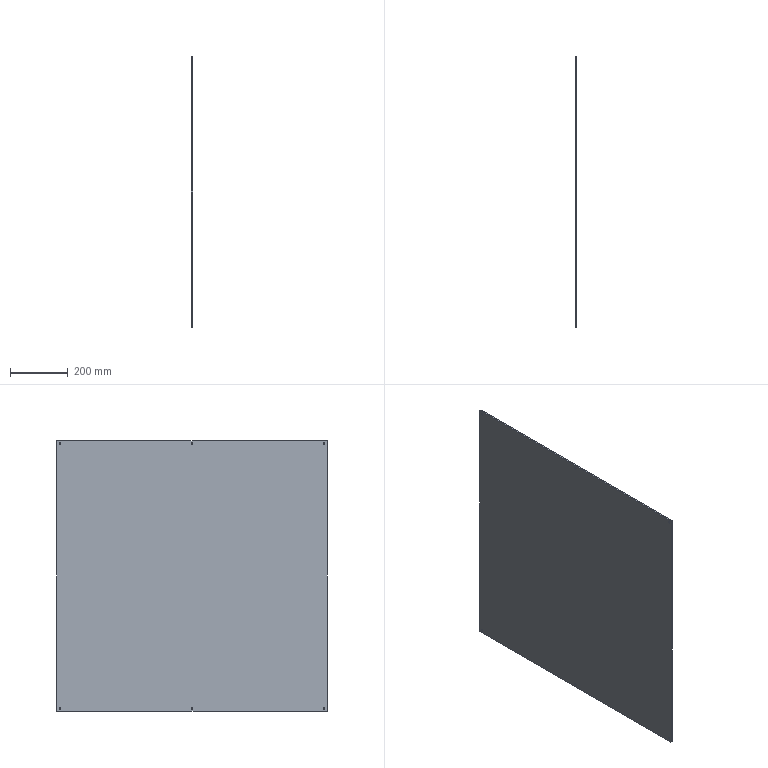Part | SolidWorks | features Chamfer 1, Extrusion 1, ICE 1 | 1 solid | 22 faces | box 5 x 937 x 938 mm | volume 4393672 mm3 | cylinder 12 | plane 10 | commonest cylinder face diameters 6 x12
STEP:
#1=CARTESIAN_POINT('',(5.,0.,-461.));
#2=VERTEX_POINT('',#1);
#3=CARTESIAN_POINT('',(5.,0.,-455.));
#4=VERTEX_POINT('',#3);
#5=CARTESIAN_POINT('',(5.,0.,-458.));
#6=DIRECTION('',(-1.,0.,0.));
#7=DIRECTION('',(0.,0.,1.));
#8=AXIS2_PLACEMENT_3D('',#5,#6,#7);
#9=CIRCLE('',#8,3.);
#10=EDGE_CURVE('',#2,#4,#9,.T.);
#11=ORIENTED_EDGE('',*,*,#10,.F.);
#12=CARTESIAN_POINT('',(0.,0.,-461.));
#13=VERTEX_POINT('',#12);
#14=CARTESIAN_POINT('',(5.,0.,-461.));
#15=DIRECTION('',(-1.,0.,0.));
#16=VECTOR('',#15,1000.);
#17=LINE('',#14,#16);
#18=EDGE_CURVE('',#2,#13,#17,.T.);
#19=ORIENTED_EDGE('',*,*,#18,.T.);
#20=CARTESIAN_POINT('',(0.,0.,-455.));
#21=VERTEX_POINT('',#20);
#22=CARTESIAN_POINT('',(0.,0.,-458.));
#23=DIRECTION('',(-1.,0.,0.));
#24=DIRECTION('',(0.,0.,1.));
#25=AXIS2_PLACEMENT_3D('',#22,#23,#24);
#26=CIRCLE('',#25,3.);
#27=EDGE_CURVE('',#13,#21,#26,.T.);
#28=ORIENTED_EDGE('',*,*,#27,.T.);
#29=CARTESIAN_POINT('',(5.,0.,-455.));
#30=DIRECTION('',(-1.,0.,0.));
#31=VECTOR('',#30,1000.);
#32=LINE('',#29,#31);
#33=EDGE_CURVE('',#4,#21,#32,.T.);
#34=ORIENTED_EDGE('',*,*,#33,.F.);
#35=EDGE_LOOP('',(#11,#19,#28,#34));
#36=FACE_OUTER_BOUND('',#35,.T.);
#37=CARTESIAN_POINT('',(5.,0.,-458.));
#38=DIRECTION('',(-1.,0.,0.));
#39=DIRECTION('',(0.,0.,1.));
#40=AXIS2_PLACEMENT_3D('',#37,#38,#39);
#41=CYLINDRICAL_SURFACE('',#40,3.);
#42=ADVANCED_FACE('',(#36),#41,.F.);
#43=CARTESIAN_POINT('',(5.,0.,455.));
#44=VERTEX_POINT('',#43);
#45=CARTESIAN_POINT('',(5.,0.,461.));
#46=VERTEX_POINT('',#45);
#47=CARTESIAN_POINT('',(5.,0.,458.));
#48=DIRECTION('',(-1.,0.,0.));
#49=DIRECTION('',(0.,0.,1.));
#50=AXIS2_PLACEMENT_3D('',#47,#48,#49);
#51=CIRCLE('',#50,3.);
#52=EDGE_CURVE('',#44,#46,#51,.T.);
#53=ORIENTED_EDGE('',*,*,#52,.F.);
#54=CARTESIAN_POINT('',(0.,0.,455.));
#55=VERTEX_POINT('',#54);
#56=CARTESIAN_POINT('',(5.,0.,455.));
#57=DIRECTION('',(-1.,0.,0.));
#58=VECTOR('',#57,1000.);
#59=LINE('',#56,#58);
#60=EDGE_CURVE('',#44,#55,#59,.T.);
#61=ORIENTED_EDGE('',*,*,#60,.T.);
#62=CARTESIAN_POINT('',(0.,0.,461.));
#63=VERTEX_POINT('',#62);
#64=CARTESIAN_POINT('',(0.,0.,458.));
#65=DIRECTION('',(-1.,0.,0.));
#66=DIRECTION('',(0.,0.,1.));
#67=AXIS2_PLACEMENT_3D('',#64,#65,#66);
#68=CIRCLE('',#67,3.);
#69=EDGE_CURVE('',#55,#63,#68,.T.);
#70=ORIENTED_EDGE('',*,*,#69,.T.);
#71=CARTESIAN_POINT('',(5.,0.,461.));
#72=DIRECTION('',(-1.,0.,0.));
#73=VECTOR('',#72,1000.);
#74=LINE('',#71,#73);
#75=EDGE_CURVE('',#46,#63,#74,.T.);
#76=ORIENTED_EDGE('',*,*,#75,.F.);
#77=EDGE_LOOP('',(#53,#61,#70,#76));
#78=FACE_OUTER_BOUND('',#77,.T.);
#79=CARTESIAN_POINT('',(5.,0.,458.));
#80=DIRECTION('',(-1.,0.,0.));
#81=DIRECTION('',(0.,0.,1.));
#82=AXIS2_PLACEMENT_3D('',#79,#80,#81);
#83=CYLINDRICAL_SURFACE('',#82,3.);
#84=ADVANCED_FACE('',(#78),#83,.F.);
#85=CARTESIAN_POINT('',(5.,457.5,455.));
#86=VERTEX_POINT('',#85);
#87=CARTESIAN_POINT('',(5.,457.5,461.));
#88=VERTEX_POINT('',#87);
#89=CARTESIAN_POINT('',(5.,457.5,458.));
#90=DIRECTION('',(-1.,0.,0.));
#91=DIRECTION('',(0.,0.,-1.));
#92=AXIS2_PLACEMENT_3D('',#89,#90,#91);
#93=CIRCLE('',#92,3.);
#94=EDGE_CURVE('',#86,#88,#93,.T.);
#95=ORIENTED_EDGE('',*,*,#94,.F.);
#96=CARTESIAN_POINT('',(0.,457.5,455.));
#97=VERTEX_POINT('',#96);
#98=CARTESIAN_POINT('',(5.,457.5,455.));
#99=DIRECTION('',(-1.,0.,0.));
#100=VECTOR('',#99,1000.);
#101=LINE('',#98,#100);
#102=EDGE_CURVE('',#86,#97,#101,.T.);
#103=ORIENTED_EDGE('',*,*,#102,.T.);
#104=CARTESIAN_POINT('',(0.,457.5,461.));
#105=VERTEX_POINT('',#104);
#106=CARTESIAN_POINT('',(0.,457.5,458.));
#107=DIRECTION('',(-1.,0.,0.));
#108=DIRECTION('',(0.,0.,-1.));
#109=AXIS2_PLACEMENT_3D('',#106,#107,#108);
#110=CIRCLE('',#109,3.);
#111=EDGE_CURVE('',#97,#105,#110,.T.);
#112=ORIENTED_EDGE('',*,*,#111,.T.);
#113=CARTESIAN_POINT('',(5.,457.5,461.));
#114=DIRECTION('',(-1.,0.,0.));
#115=VECTOR('',#114,1000.);
#116=LINE('',#113,#115);
#117=EDGE_CURVE('',#88,#105,#116,.T.);
#118=ORIENTED_EDGE('',*,*,#117,.F.);
#119=EDGE_LOOP('',(#95,#103,#112,#118));
#120=FACE_OUTER_BOUND('',#119,.T.);
#121=CARTESIAN_POINT('',(5.,457.5,458.));
#122=DIRECTION('',(-1.,0.,0.));
#123=DIRECTION('',(0.,0.,1.));
#124=AXIS2_PLACEMENT_3D('',#121,#122,#123);
#125=CYLINDRICAL_SURFACE('',#124,3.);
#126=ADVANCED_FACE('',(#120),#125,.F.);
#127=CARTESIAN_POINT('',(5.,-457.5,455.));
#128=VERTEX_POINT('',#127);
#129=CARTESIAN_POINT('',(5.,-457.5,461.));
#130=VERTEX_POINT('',#129);
#131=CARTESIAN_POINT('',(5.,-457.5,458.));
#132=DIRECTION('',(-1.,0.,0.));
#133=DIRECTION('',(0.,0.,1.));
#134=AXIS2_PLACEMENT_3D('',#131,#132,#133);
#135=CIRCLE('',#134,3.);
#136=EDGE_CURVE('',#128,#130,#135,.T.);
#137=ORIENTED_EDGE('',*,*,#136,.F.);
#138=CARTESIAN_POINT('',(0.,-457.5,455.));
#139=VERTEX_POINT('',#138);
#140=CARTESIAN_POINT('',(5.,-457.5,455.));
#141=DIRECTION('',(-1.,0.,0.));
#142=VECTOR('',#141,1000.);
#143=LINE('',#140,#142);
#144=EDGE_CURVE('',#128,#139,#143,.T.);
#145=ORIENTED_EDGE('',*,*,#144,.T.);
#146=CARTESIAN_POINT('',(0.,-457.5,461.));
#147=VERTEX_POINT('',#146);
#148=CARTESIAN_POINT('',(0.,-457.5,458.));
#149=DIRECTION('',(-1.,0.,0.));
#150=DIRECTION('',(0.,0.,1.));
#151=AXIS2_PLACEMENT_3D('',#148,#149,#150);
#152=CIRCLE('',#151,3.);
#153=EDGE_CURVE('',#139,#147,#152,.T.);
#154=ORIENTED_EDGE('',*,*,#153,.T.);
#155=CARTESIAN_POINT('',(5.,-457.5,461.));
#156=DIRECTION('',(-1.,0.,0.));
#157=VECTOR('',#156,1000.);
#158=LINE('',#155,#157);
#159=EDGE_CURVE('',#130,#147,#158,.T.);
#160=ORIENTED_EDGE('',*,*,#159,.F.);
#161=EDGE_LOOP('',(#137,#145,#154,#160));
#162=FACE_OUTER_BOUND('',#161,.T.);
#163=CARTESIAN_POINT('',(5.,-457.5,458.));
#164=DIRECTION('',(-1.,0.,0.));
#165=DIRECTION('',(0.,0.,1.));
#166=AXIS2_PLACEMENT_3D('',#163,#164,#165);
#167=CYLINDRICAL_SURFACE('',#166,3.);
#168=ADVANCED_FACE('',(#162),#167,.F.);
#169=CARTESIAN_POINT('',(5.,-457.5,-461.));
#170=VERTEX_POINT('',#169);
#171=CARTESIAN_POINT('',(5.,-457.5,-455.));
#172=VERTEX_POINT('',#171);
#173=CARTESIAN_POINT('',(5.,-457.5,-458.));
#174=DIRECTION('',(-1.,0.,0.));
#175=DIRECTION('',(0.,0.,-1.));
#176=AXIS2_PLACEMENT_3D('',#173,#174,#175);
#177=CIRCLE('',#176,3.);
#178=EDGE_CURVE('',#170,#172,#177,.T.);
#179=ORIENTED_EDGE('',*,*,#178,.F.);
#180=CARTESIAN_POINT('',(0.,-457.5,-461.));
#181=VERTEX_POINT('',#180);
#182=CARTESIAN_POINT('',(5.,-457.5,-461.));
#183=DIRECTION('',(-1.,0.,0.));
#184=VECTOR('',#183,1000.);
#185=LINE('',#182,#184);
#186=EDGE_CURVE('',#170,#181,#185,.T.);
#187=ORIENTED_EDGE('',*,*,#186,.T.);
#188=CARTESIAN_POINT('',(0.,-457.5,-455.));
#189=VERTEX_POINT('',#188);
#190=CARTESIAN_POINT('',(0.,-457.5,-458.));
#191=DIRECTION('',(-1.,0.,0.));
#192=DIRECTION('',(0.,0.,-1.));
#193=AXIS2_PLACEMENT_3D('',#190,#191,#192);
#194=CIRCLE('',#193,3.);
#195=EDGE_CURVE('',#181,#189,#194,.T.);
#196=ORIENTED_EDGE('',*,*,#195,.T.);
#197=CARTESIAN_POINT('',(5.,-457.5,-455.));
#198=DIRECTION('',(-1.,0.,0.));
#199=VECTOR('',#198,1000.);
#200=LINE('',#197,#199);
#201=EDGE_CURVE('',#172,#189,#200,.T.);
#202=ORIENTED_EDGE('',*,*,#201,.F.);
#203=EDGE_LOOP('',(#179,#187,#196,#202));
#204=FACE_OUTER_BOUND('',#203,.T.);
#205=CARTESIAN_POINT('',(5.,-457.5,-458.));
#206=DIRECTION('',(-1.,0.,0.));
#207=DIRECTION('',(0.,0.,1.));
#208=AXIS2_PLACEMENT_3D('',#205,#206,#207);
#209=CYLINDRICAL_SURFACE('',#208,3.);
#210=ADVANCED_FACE('',(#204),#209,.F.);
#211=CARTESIAN_POINT('',(5.,457.5,-461.));
#212=VERTEX_POINT('',#211);
#213=CARTESIAN_POINT('',(5.,457.5,-455.));
#214=VERTEX_POINT('',#213);
#215=CARTESIAN_POINT('',(5.,457.5,-458.));
#216=DIRECTION('',(-1.,0.,0.));
#217=DIRECTION('',(0.,0.,1.));
#218=AXIS2_PLACEMENT_3D('',#215,#216,#217);
#219=CIRCLE('',#218,3.);
#220=EDGE_CURVE('',#212,#214,#219,.T.);
#221=ORIENTED_EDGE('',*,*,#220,.F.);
#222=CARTESIAN_POINT('',(0.,457.5,-461.));
#223=VERTEX_POINT('',#222);
#224=CARTESIAN_POINT('',(5.,457.5,-461.));
#225=DIRECTION('',(-1.,0.,0.));
#226=VECTOR('',#225,1000.);
#227=LINE('',#224,#226);
#228=EDGE_CURVE('',#212,#223,#227,.T.);
#229=ORIENTED_EDGE('',*,*,#228,.T.);
#230=CARTESIAN_POINT('',(0.,457.5,-455.));
#231=VERTEX_POINT('',#230);
#232=CARTESIAN_POINT('',(0.,457.5,-458.));
#233=DIRECTION('',(-1.,0.,0.));
#234=DIRECTION('',(0.,0.,1.));
#235=AXIS2_PLACEMENT_3D('',#232,#233,#234);
#236=CIRCLE('',#235,3.);
#237=EDGE_CURVE('',#223,#231,#236,.T.);
#238=ORIENTED_EDGE('',*,*,#237,.T.);
#239=CARTESIAN_POINT('',(5.,457.5,-455.));
#240=DIRECTION('',(-1.,0.,0.));
#241=VECTOR('',#240,1000.);
#242=LINE('',#239,#241);
#243=EDGE_CURVE('',#214,#231,#242,.T.);
#244=ORIENTED_EDGE('',*,*,#243,.F.);
#245=EDGE_LOOP('',(#221,#229,#238,#244));
#246=FACE_OUTER_BOUND('',#245,.T.);
#247=CARTESIAN_POINT('',(5.,457.5,-458.));
#248=DIRECTION('',(-1.,0.,0.));
#249=DIRECTION('',(0.,0.,1.));
#250=AXIS2_PLACEMENT_3D('',#247,#248,#249);
#251=CYLINDRICAL_SURFACE('',#250,3.);
#252=ADVANCED_FACE('',(#246),#251,.F.);
#253=CARTESIAN_POINT('',(0.,467.5,469.));
#254=VERTEX_POINT('',#253);
#255=CARTESIAN_POINT('',(0.,-467.5,469.));
#256=VERTEX_POINT('',#255);
#257=CARTESIAN_POINT('',(0.,468.5,469.));
#258=DIRECTION('',(0.,-1.,0.));
#259=VECTOR('',#258,1000.);
#260=LINE('',#257,#259);
#261=EDGE_CURVE('',#254,#256,#260,.T.);
#262=ORIENTED_EDGE('',*,*,#261,.T.);
#263=CARTESIAN_POINT('',(5.,-467.5,469.));
#264=VERTEX_POINT('',#263);
#265=CARTESIAN_POINT('',(5.,-467.5,469.));
#266=DIRECTION('',(1.,0.,0.));
#267=VECTOR('',#266,1000.);
#268=LINE('',#265,#267);
#269=EDGE_CURVE('',#256,#264,#268,.T.);
#270=ORIENTED_EDGE('',*,*,#269,.T.);
#271=CARTESIAN_POINT('',(5.,467.5,469.));
#272=VERTEX_POINT('',#271);
#273=CARTESIAN_POINT('',(5.,468.5,469.));
#274=DIRECTION('',(0.,-1.,0.));
#275=VECTOR('',#274,1000.);
#276=LINE('',#273,#275);
#277=EDGE_CURVE('',#272,#264,#276,.T.);
#278=ORIENTED_EDGE('',*,*,#277,.F.);
#279=CARTESIAN_POINT('',(5.,467.5,469.));
#280=DIRECTION('',(-1.,0.,0.));
#281=VECTOR('',#280,1000.);
#282=LINE('',#279,#281);
#283=EDGE_CURVE('',#272,#254,#282,.T.);
#284=ORIENTED_EDGE('',*,*,#283,.T.);
#285=EDGE_LOOP('',(#262,#270,#278,#284));
#286=FACE_OUTER_BOUND('',#285,.T.);
#287=CARTESIAN_POINT('',(5.,468.5,469.));
#288=DIRECTION('',(0.,0.,-1.));
#289=DIRECTION('',(0.,1.,0.));
#290=AXIS2_PLACEMENT_3D('',#287,#288,#289);
#291=PLANE('',#290);
#292=ADVANCED_FACE('',(#286),#291,.F.);
#293=CARTESIAN_POINT('',(0.,-468.5,468.));
#294=VERTEX_POINT('',#293);
#295=CARTESIAN_POINT('',(0.,-468.5,-468.));
#296=VERTEX_POINT('',#295);
#297=CARTESIAN_POINT('',(0.,-468.5,-469.));
#298=DIRECTION('',(0.,0.,-1.));
#299=VECTOR('',#298,1000.);
#300=LINE('',#297,#299);
#301=EDGE_CURVE('',#294,#296,#300,.T.);
#302=ORIENTED_EDGE('',*,*,#301,.T.);
#303=CARTESIAN_POINT('',(5.,-468.5,-468.));
#304=VERTEX_POINT('',#303);
#305=CARTESIAN_POINT('',(5.,-468.5,-468.));
#306=DIRECTION('',(1.,0.,0.));
#307=VECTOR('',#306,1000.);
#308=LINE('',#305,#307);
#309=EDGE_CURVE('',#296,#304,#308,.T.);
#310=ORIENTED_EDGE('',*,*,#309,.T.);
#311=CARTESIAN_POINT('',(5.,-468.5,468.));
#312=VERTEX_POINT('',#311);
#313=CARTESIAN_POINT('',(5.,-468.5,-469.));
#314=DIRECTION('',(0.,0.,-1.));
#315=VECTOR('',#314,1000.);
#316=LINE('',#313,#315);
#317=EDGE_CURVE('',#312,#304,#316,.T.);
#318=ORIENTED_EDGE('',*,*,#317,.F.);
#319=CARTESIAN_POINT('',(5.,-468.5,468.));
#320=DIRECTION('',(-1.,0.,0.));
#321=VECTOR('',#320,1000.);
#322=LINE('',#319,#321);
#323=EDGE_CURVE('',#312,#294,#322,.T.);
#324=ORIENTED_EDGE('',*,*,#323,.T.);
#325=EDGE_LOOP('',(#302,#310,#318,#324));
#326=FACE_OUTER_BOUND('',#325,.T.);
#327=CARTESIAN_POINT('',(5.,-468.5,-469.));
#328=DIRECTION('',(0.,1.,0.));
#329=DIRECTION('',(0.,0.,1.));
#330=AXIS2_PLACEMENT_3D('',#327,#328,#329);
#331=PLANE('',#330);
#332=ADVANCED_FACE('',(#326),#331,.F.);
#333=CARTESIAN_POINT('',(5.,-467.5,-469.));
#334=VERTEX_POINT('',#333);
#335=CARTESIAN_POINT('',(5.,467.5,-469.));
#336=VERTEX_POINT('',#335);
#337=CARTESIAN_POINT('',(5.,468.5,-469.));
#338=DIRECTION('',(0.,1.,0.));
#339=VECTOR('',#338,1000.);
#340=LINE('',#337,#339);
#341=EDGE_CURVE('',#334,#336,#340,.T.);
#342=ORIENTED_EDGE('',*,*,#341,.F.);
#343=CARTESIAN_POINT('',(0.,-467.5,-469.));
#344=VERTEX_POINT('',#343);
#345=CARTESIAN_POINT('',(5.,-467.5,-469.));
#346=DIRECTION('',(-1.,0.,0.));
#347=VECTOR('',#346,1000.);
#348=LINE('',#345,#347);
#349=EDGE_CURVE('',#334,#344,#348,.T.);
#350=ORIENTED_EDGE('',*,*,#349,.T.);
#351=CARTESIAN_POINT('',(0.,467.5,-469.));
#352=VERTEX_POINT('',#351);
#353=CARTESIAN_POINT('',(0.,468.5,-469.));
#354=DIRECTION('',(0.,1.,0.));
#355=VECTOR('',#354,1000.);
#356=LINE('',#353,#355);
#357=EDGE_CURVE('',#344,#352,#356,.T.);
#358=ORIENTED_EDGE('',*,*,#357,.T.);
#359=CARTESIAN_POINT('',(5.,467.5,-469.));
#360=DIRECTION('',(1.,0.,0.));
#361=VECTOR('',#360,1000.);
#362=LINE('',#359,#361);
#363=EDGE_CURVE('',#352,#336,#362,.T.);
#364=ORIENTED_EDGE('',*,*,#363,.T.);
#365=EDGE_LOOP('',(#342,#350,#358,#364));
#366=FACE_OUTER_BOUND('',#365,.T.);
#367=CARTESIAN_POINT('',(5.,468.5,-469.));
#368=DIRECTION('',(0.,0.,1.));
#369=DIRECTION('',(0.,-1.,0.));
#370=AXIS2_PLACEMENT_3D('',#367,#368,#369);
#371=PLANE('',#370);
#372=ADVANCED_FACE('',(#366),#371,.F.);
#373=CARTESIAN_POINT('',(5.,468.5,-468.));
#374=VERTEX_POINT('',#373);
#375=CARTESIAN_POINT('',(5.,468.5,468.));
#376=VERTEX_POINT('',#375);
#377=CARTESIAN_POINT('',(5.,468.5,-469.));
#378=DIRECTION('',(0.,0.,1.));
#379=VECTOR('',#378,1000.);
#380=LINE('',#377,#379);
#381=EDGE_CURVE('',#374,#376,#380,.T.);
#382=ORIENTED_EDGE('',*,*,#381,.F.);
#383=CARTESIAN_POINT('',(0.,468.5,-468.));
#384=VERTEX_POINT('',#383);
#385=CARTESIAN_POINT('',(5.,468.5,-468.));
#386=DIRECTION('',(-1.,0.,0.));
#387=VECTOR('',#386,1000.);
#388=LINE('',#385,#387);
#389=EDGE_CURVE('',#374,#384,#388,.T.);
#390=ORIENTED_EDGE('',*,*,#389,.T.);
#391=CARTESIAN_POINT('',(0.,468.5,468.));
#392=VERTEX_POINT('',#391);
#393=CARTESIAN_POINT('',(0.,468.5,-469.));
#394=DIRECTION('',(0.,0.,1.));
#395=VECTOR('',#394,1000.);
#396=LINE('',#393,#395);
#397=EDGE_CURVE('',#384,#392,#396,.T.);
#398=ORIENTED_EDGE('',*,*,#397,.T.);
#399=CARTESIAN_POINT('',(5.,468.5,468.));
#400=DIRECTION('',(1.,0.,0.));
#401=VECTOR('',#400,1000.);
#402=LINE('',#399,#401);
#403=EDGE_CURVE('',#392,#376,#402,.T.);
#404=ORIENTED_EDGE('',*,*,#403,.T.);
#405=EDGE_LOOP('',(#382,#390,#398,#404));
#406=FACE_OUTER_BOUND('',#405,.T.);
#407=CARTESIAN_POINT('',(5.,468.5,-469.));
#408=DIRECTION('',(0.,-1.,0.));
#409=DIRECTION('',(0.,0.,-1.));
#410=AXIS2_PLACEMENT_3D('',#407,#408,#409);
#411=PLANE('',#410);
#412=ADVANCED_FACE('',(#406),#411,.F.);
#413=CARTESIAN_POINT('',(5.,0.,-458.));
#414=DIRECTION('',(-1.,0.,0.));
#415=DIRECTION('',(0.,0.,1.));
#416=AXIS2_PLACEMENT_3D('',#413,#414,#415);
#417=CIRCLE('',#416,3.);
#418=EDGE_CURVE('',#4,#2,#417,.T.);
#419=ORIENTED_EDGE('',*,*,#418,.T.);
#420=ORIENTED_EDGE('',*,*,#10,.T.);
#421=EDGE_LOOP('',(#419,#420));
#422=FACE_BOUND('',#421,.T.);
#423=CARTESIAN_POINT('',(5.,0.,458.));
#424=DIRECTION('',(-1.,0.,0.));
#425=DIRECTION('',(0.,0.,1.));
#426=AXIS2_PLACEMENT_3D('',#423,#424,#425);
#427=CIRCLE('',#426,3.);
#428=EDGE_CURVE('',#46,#44,#427,.T.);
#429=ORIENTED_EDGE('',*,*,#428,.T.);
#430=ORIENTED_EDGE('',*,*,#52,.T.);
#431=EDGE_LOOP('',(#429,#430));
#432=FACE_BOUND('',#431,.T.);
#433=CARTESIAN_POINT('',(5.,457.5,458.));
#434=DIRECTION('',(-1.,0.,0.));
#435=DIRECTION('',(0.,0.,-1.));
#436=AXIS2_PLACEMENT_3D('',#433,#434,#435);
#437=CIRCLE('',#436,3.);
#438=EDGE_CURVE('',#88,#86,#437,.T.);
#439=ORIENTED_EDGE('',*,*,#438,.T.);
#440=ORIENTED_EDGE('',*,*,#94,.T.);
#441=EDGE_LOOP('',(#439,#440));
#442=FACE_BOUND('',#441,.T.);
#443=CARTESIAN_POINT('',(5.,-457.5,458.));
#444=DIRECTION('',(-1.,0.,0.));
#445=DIRECTION('',(0.,0.,1.));
#446=AXIS2_PLACEMENT_3D('',#443,#444,#445);
#447=CIRCLE('',#446,3.);
#448=EDGE_CURVE('',#130,#128,#447,.T.);
#449=ORIENTED_EDGE('',*,*,#448,.T.);
#450=ORIENTED_EDGE('',*,*,#136,.T.);
#451=EDGE_LOOP('',(#449,#450));
#452=FACE_BOUND('',#451,.T.);
#453=CARTESIAN_POINT('',(5.,-457.5,-458.));
#454=DIRECTION('',(-1.,0.,0.));
#455=DIRECTION('',(0.,0.,-1.));
#456=AXIS2_PLACEMENT_3D('',#453,#454,#455);
#457=CIRCLE('',#456,3.);
#458=EDGE_CURVE('',#172,#170,#457,.T.);
#459=ORIENTED_EDGE('',*,*,#458,.T.);
#460=ORIENTED_EDGE('',*,*,#178,.T.);
#461=EDGE_LOOP('',(#459,#460));
#462=FACE_BOUND('',#461,.T.);
#463=CARTESIAN_POINT('',(5.,457.5,-458.));
#464=DIRECTION('',(-1.,0.,0.));
#465=DIRECTION('',(0.,0.,1.));
#466=AXIS2_PLACEMENT_3D('',#463,#464,#465);
#467=CIRCLE('',#466,3.);
#468=EDGE_CURVE('',#214,#212,#467,.T.);
#469=ORIENTED_EDGE('',*,*,#468,.T.);
#470=ORIENTED_EDGE('',*,*,#220,.T.);
#471=EDGE_LOOP('',(#469,#470));
#472=FACE_BOUND('',#471,.T.);
#473=ORIENTED_EDGE('',*,*,#317,.T.);
#474=CARTESIAN_POINT('',(5.,-467.5,-469.));
#475=DIRECTION('',(0.,0.7071,-0.7071));
#476=VECTOR('',#475,1000.);
#477=LINE('',#474,#476);
#478=EDGE_CURVE('',#304,#334,#477,.T.);
#479=ORIENTED_EDGE('',*,*,#478,.T.);
#480=ORIENTED_EDGE('',*,*,#341,.T.);
#481=CARTESIAN_POINT('',(5.,468.5,-468.));
#482=DIRECTION('',(0.,0.7071,0.7071));
#483=VECTOR('',#482,1000.);
#484=LINE('',#481,#483);
#485=EDGE_CURVE('',#336,#374,#484,.T.);
#486=ORIENTED_EDGE('',*,*,#485,.T.);
#487=ORIENTED_EDGE('',*,*,#381,.T.);
#488=CARTESIAN_POINT('',(5.,467.5,469.));
#489=DIRECTION('',(0.,-0.7071,0.7071));
#490=VECTOR('',#489,1000.);
#491=LINE('',#488,#490);
#492=EDGE_CURVE('',#376,#272,#491,.T.);
#493=ORIENTED_EDGE('',*,*,#492,.T.);
#494=ORIENTED_EDGE('',*,*,#277,.T.);
#495=CARTESIAN_POINT('',(5.,-468.5,468.));
#496=DIRECTION('',(0.,-0.7071,-0.7071));
#497=VECTOR('',#496,1000.);
#498=LINE('',#495,#497);
#499=EDGE_CURVE('',#264,#312,#498,.T.);
#500=ORIENTED_EDGE('',*,*,#499,.T.);
#501=EDGE_LOOP('',(#473,#479,#480,#486,#487,#493,#494,#500));
#502=FACE_OUTER_BOUND('',#501,.T.);
#503=CARTESIAN_POINT('',(5.,-468.5,469.));
#504=DIRECTION('',(-1.,0.,0.));
#505=DIRECTION('',(0.,0.,1.));
#506=AXIS2_PLACEMENT_3D('',#503,#504,#505);
#507=PLANE('',#506);
#508=ADVANCED_FACE('',(#422,#432,#442,#452,#462,#472,#502),#507,.F.);
#509=CARTESIAN_POINT('',(0.,0.,-458.));
#510=DIRECTION('',(-1.,0.,0.));
#511=DIRECTION('',(0.,0.,1.));
#512=AXIS2_PLACEMENT_3D('',#509,#510,#511);
#513=CIRCLE('',#512,3.);
#514=EDGE_CURVE('',#21,#13,#513,.T.);
#515=ORIENTED_EDGE('',*,*,#514,.F.);
#516=ORIENTED_EDGE('',*,*,#27,.F.);
#517=EDGE_LOOP('',(#515,#516));
#518=FACE_BOUND('',#517,.T.);
#519=CARTESIAN_POINT('',(0.,0.,458.));
#520=DIRECTION('',(-1.,0.,0.));
#521=DIRECTION('',(0.,0.,1.));
#522=AXIS2_PLACEMENT_3D('',#519,#520,#521);
#523=CIRCLE('',#522,3.);
#524=EDGE_CURVE('',#63,#55,#523,.T.);
#525=ORIENTED_EDGE('',*,*,#524,.F.);
#526=ORIENTED_EDGE('',*,*,#69,.F.);
#527=EDGE_LOOP('',(#525,#526));
#528=FACE_BOUND('',#527,.T.);
#529=CARTESIAN_POINT('',(0.,457.5,458.));
#530=DIRECTION('',(-1.,0.,0.));
#531=DIRECTION('',(0.,0.,-1.));
#532=AXIS2_PLACEMENT_3D('',#529,#530,#531);
#533=CIRCLE('',#532,3.);
#534=EDGE_CURVE('',#105,#97,#533,.T.);
#535=ORIENTED_EDGE('',*,*,#534,.F.);
#536=ORIENTED_EDGE('',*,*,#111,.F.);
#537=EDGE_LOOP('',(#535,#536));
#538=FACE_BOUND('',#537,.T.);
#539=CARTESIAN_POINT('',(0.,-457.5,458.));
#540=DIRECTION('',(-1.,0.,0.));
#541=DIRECTION('',(0.,0.,1.));
#542=AXIS2_PLACEMENT_3D('',#539,#540,#541);
#543=CIRCLE('',#542,3.);
#544=EDGE_CURVE('',#147,#139,#543,.T.);
#545=ORIENTED_EDGE('',*,*,#544,.F.);
#546=ORIENTED_EDGE('',*,*,#153,.F.);
#547=EDGE_LOOP('',(#545,#546));
#548=FACE_BOUND('',#547,.T.);
#549=CARTESIAN_POINT('',(0.,-457.5,-458.));
#550=DIRECTION('',(-1.,0.,0.));
#551=DIRECTION('',(0.,0.,-1.));
#552=AXIS2_PLACEMENT_3D('',#549,#550,#551);
#553=CIRCLE('',#552,3.);
#554=EDGE_CURVE('',#189,#181,#553,.T.);
#555=ORIENTED_EDGE('',*,*,#554,.F.);
#556=ORIENTED_EDGE('',*,*,#195,.F.);
#557=EDGE_LOOP('',(#555,#556));
#558=FACE_BOUND('',#557,.T.);
#559=CARTESIAN_POINT('',(0.,457.5,-458.));
#560=DIRECTION('',(-1.,0.,0.));
#561=DIRECTION('',(0.,0.,1.));
#562=AXIS2_PLACEMENT_3D('',#559,#560,#561);
#563=CIRCLE('',#562,3.);
#564=EDGE_CURVE('',#231,#223,#563,.T.);
#565=ORIENTED_EDGE('',*,*,#564,.F.);
#566=ORIENTED_EDGE('',*,*,#237,.F.);
#567=EDGE_LOOP('',(#565,#566));
#568=FACE_BOUND('',#567,.T.);
#569=ORIENTED_EDGE('',*,*,#357,.F.);
#570=CARTESIAN_POINT('',(0.,-937.,0.5));
#571=DIRECTION('',(0.,-0.7071,0.7071));
#572=VECTOR('',#571,1000.);
#573=LINE('',#570,#572);
#574=EDGE_CURVE('',#344,#296,#573,.T.);
#575=ORIENTED_EDGE('',*,*,#574,.T.);
#576=ORIENTED_EDGE('',*,*,#301,.F.);
#577=CARTESIAN_POINT('',(0.,-468.,468.5));
#578=DIRECTION('',(0.,0.7071,0.7071));
#579=VECTOR('',#578,1000.);
#580=LINE('',#577,#579);
#581=EDGE_CURVE('',#294,#256,#580,.T.);
#582=ORIENTED_EDGE('',*,*,#581,.T.);
#583=ORIENTED_EDGE('',*,*,#261,.F.);
#584=CARTESIAN_POINT('',(0.,-0.5,937.));
#585=DIRECTION('',(0.,0.7071,-0.7071));
#586=VECTOR('',#585,1000.);
#587=LINE('',#584,#586);
#588=EDGE_CURVE('',#254,#392,#587,.T.);
#589=ORIENTED_EDGE('',*,*,#588,.T.);
#590=ORIENTED_EDGE('',*,*,#397,.F.);
#591=CARTESIAN_POINT('',(0.,468.5,-468.));
#592=DIRECTION('',(0.,-0.7071,-0.7071));
#593=VECTOR('',#592,1000.);
#594=LINE('',#591,#593);
#595=EDGE_CURVE('',#384,#352,#594,.T.);
#596=ORIENTED_EDGE('',*,*,#595,.T.);
#597=EDGE_LOOP('',(#569,#575,#576,#582,#583,#589,#590,#596));
#598=FACE_OUTER_BOUND('',#597,.T.);
#599=CARTESIAN_POINT('',(0.,-468.5,469.));
#600=DIRECTION('',(-1.,0.,0.));
#601=DIRECTION('',(0.,0.,1.));
#602=AXIS2_PLACEMENT_3D('',#599,#600,#601);
#603=PLANE('',#602);
#604=ADVANCED_FACE('',(#518,#528,#538,#548,#558,#568,#598),#603,.T.);
#605=ORIENTED_EDGE('',*,*,#478,.F.);
#606=ORIENTED_EDGE('',*,*,#309,.F.);
#607=ORIENTED_EDGE('',*,*,#574,.F.);
#608=ORIENTED_EDGE('',*,*,#349,.F.);
#609=EDGE_LOOP('',(#605,#606,#607,#608));
#610=FACE_OUTER_BOUND('',#609,.T.);
#611=CARTESIAN_POINT('',(5.,-467.5,-469.));
#612=DIRECTION('',(0.,0.7071,0.7071));
#613=DIRECTION('',(0.,-0.7071,0.7071));
#614=AXIS2_PLACEMENT_3D('',#611,#612,#613);
#615=PLANE('',#614);
#616=ADVANCED_FACE('',(#610),#615,.F.);
#617=ORIENTED_EDGE('',*,*,#499,.F.);
#618=ORIENTED_EDGE('',*,*,#269,.F.);
#619=ORIENTED_EDGE('',*,*,#581,.F.);
#620=ORIENTED_EDGE('',*,*,#323,.F.);
#621=EDGE_LOOP('',(#617,#618,#619,#620));
#622=FACE_OUTER_BOUND('',#621,.T.);
#623=CARTESIAN_POINT('',(5.,-468.5,468.));
#624=DIRECTION('',(0.,0.7071,-0.7071));
#625=DIRECTION('',(0.,0.7071,0.7071));
#626=AXIS2_PLACEMENT_3D('',#623,#624,#625);
#627=PLANE('',#626);
#628=ADVANCED_FACE('',(#622),#627,.F.);
#629=ORIENTED_EDGE('',*,*,#485,.F.);
#630=ORIENTED_EDGE('',*,*,#363,.F.);
#631=ORIENTED_EDGE('',*,*,#595,.F.);
#632=ORIENTED_EDGE('',*,*,#389,.F.);
#633=EDGE_LOOP('',(#629,#630,#631,#632));
#634=FACE_OUTER_BOUND('',#633,.T.);
#635=CARTESIAN_POINT('',(5.,468.5,-468.));
#636=DIRECTION('',(0.,-0.7071,0.7071));
#637=DIRECTION('',(0.,-0.7071,-0.7071));
#638=AXIS2_PLACEMENT_3D('',#635,#636,#637);
#639=PLANE('',#638);
#640=ADVANCED_FACE('',(#634),#639,.F.);
#641=ORIENTED_EDGE('',*,*,#492,.F.);
#642=ORIENTED_EDGE('',*,*,#403,.F.);
#643=ORIENTED_EDGE('',*,*,#588,.F.);
#644=ORIENTED_EDGE('',*,*,#283,.F.);
#645=EDGE_LOOP('',(#641,#642,#643,#644));
#646=FACE_OUTER_BOUND('',#645,.T.);
#647=CARTESIAN_POINT('',(5.,467.5,469.));
#648=DIRECTION('',(0.,-0.7071,-0.7071));
#649=DIRECTION('',(0.,0.7071,-0.7071));
#650=AXIS2_PLACEMENT_3D('',#647,#648,#649);
#651=PLANE('',#650);
#652=ADVANCED_FACE('',(#646),#651,.F.);
#653=ORIENTED_EDGE('',*,*,#228,.F.);
#654=ORIENTED_EDGE('',*,*,#468,.F.);
#655=ORIENTED_EDGE('',*,*,#243,.T.);
#656=ORIENTED_EDGE('',*,*,#564,.T.);
#657=EDGE_LOOP('',(#653,#654,#655,#656));
#658=FACE_OUTER_BOUND('',#657,.T.);
#659=CARTESIAN_POINT('',(5.,457.5,-458.));
#660=DIRECTION('',(-1.,0.,0.));
#661=DIRECTION('',(0.,0.,1.));
#662=AXIS2_PLACEMENT_3D('',#659,#660,#661);
#663=CYLINDRICAL_SURFACE('',#662,3.);
#664=ADVANCED_FACE('',(#658),#663,.F.);
#665=ORIENTED_EDGE('',*,*,#186,.F.);
#666=ORIENTED_EDGE('',*,*,#458,.F.);
#667=ORIENTED_EDGE('',*,*,#201,.T.);
#668=ORIENTED_EDGE('',*,*,#554,.T.);
#669=EDGE_LOOP('',(#665,#666,#667,#668));
#670=FACE_OUTER_BOUND('',#669,.T.);
#671=CARTESIAN_POINT('',(5.,-457.5,-458.));
#672=DIRECTION('',(-1.,0.,0.));
#673=DIRECTION('',(0.,0.,1.));
#674=AXIS2_PLACEMENT_3D('',#671,#672,#673);
#675=CYLINDRICAL_SURFACE('',#674,3.);
#676=ADVANCED_FACE('',(#670),#675,.F.);
#677=ORIENTED_EDGE('',*,*,#144,.F.);
#678=ORIENTED_EDGE('',*,*,#448,.F.);
#679=ORIENTED_EDGE('',*,*,#159,.T.);
#680=ORIENTED_EDGE('',*,*,#544,.T.);
#681=EDGE_LOOP('',(#677,#678,#679,#680));
#682=FACE_OUTER_BOUND('',#681,.T.);
#683=CARTESIAN_POINT('',(5.,-457.5,458.));
#684=DIRECTION('',(-1.,0.,0.));
#685=DIRECTION('',(0.,0.,1.));
#686=AXIS2_PLACEMENT_3D('',#683,#684,#685);
#687=CYLINDRICAL_SURFACE('',#686,3.);
#688=ADVANCED_FACE('',(#682),#687,.F.);
#689=ORIENTED_EDGE('',*,*,#102,.F.);
#690=ORIENTED_EDGE('',*,*,#438,.F.);
#691=ORIENTED_EDGE('',*,*,#117,.T.);
#692=ORIENTED_EDGE('',*,*,#534,.T.);
#693=EDGE_LOOP('',(#689,#690,#691,#692));
#694=FACE_OUTER_BOUND('',#693,.T.);
#695=CARTESIAN_POINT('',(5.,457.5,458.));
#696=DIRECTION('',(-1.,0.,0.));
#697=DIRECTION('',(0.,0.,1.));
#698=AXIS2_PLACEMENT_3D('',#695,#696,#697);
#699=CYLINDRICAL_SURFACE('',#698,3.);
#700=ADVANCED_FACE('',(#694),#699,.F.);
#701=ORIENTED_EDGE('',*,*,#60,.F.);
#702=ORIENTED_EDGE('',*,*,#428,.F.);
#703=ORIENTED_EDGE('',*,*,#75,.T.);
#704=ORIENTED_EDGE('',*,*,#524,.T.);
#705=EDGE_LOOP('',(#701,#702,#703,#704));
#706=FACE_OUTER_BOUND('',#705,.T.);
#707=CARTESIAN_POINT('',(5.,0.,458.));
#708=DIRECTION('',(-1.,0.,0.));
#709=DIRECTION('',(0.,0.,1.));
#710=AXIS2_PLACEMENT_3D('',#707,#708,#709);
#711=CYLINDRICAL_SURFACE('',#710,3.);
#712=ADVANCED_FACE('',(#706),#711,.F.);
#713=ORIENTED_EDGE('',*,*,#18,.F.);
#714=ORIENTED_EDGE('',*,*,#418,.F.);
#715=ORIENTED_EDGE('',*,*,#33,.T.);
#716=ORIENTED_EDGE('',*,*,#514,.T.);
#717=EDGE_LOOP('',(#713,#714,#715,#716));
#718=FACE_OUTER_BOUND('',#717,.T.);
#719=CARTESIAN_POINT('',(5.,0.,-458.));
#720=DIRECTION('',(-1.,0.,0.));
#721=DIRECTION('',(0.,0.,1.));
#722=AXIS2_PLACEMENT_3D('',#719,#720,#721);
#723=CYLINDRICAL_SURFACE('',#722,3.);
#724=ADVANCED_FACE('',(#718),#723,.F.);
#725=CLOSED_SHELL('',(#42,#84,#126,#168,#210,#252,#292,#332,#372,#412,#508,#604,#616,#628,#640,#652,#664,#676,#688,#700,#712,#724));
#726=MANIFOLD_SOLID_BREP('',#725);
#727=CARTESIAN_POINT('',(0.,0.,0.));
#728=DIRECTION('',(0.,0.,1.));
#729=DIRECTION('',(1.,0.,0.));
#730=AXIS2_PLACEMENT_3D('',#727,#728,#729);
#731=(LENGTH_UNIT()NAMED_UNIT(*)SI_UNIT(.MILLI.,.METRE.));
#732=UNCERTAINTY_MEASURE_WITH_UNIT(LENGTH_MEASURE(0.00001),#731,'','');
#733=(NAMED_UNIT(*)PLANE_ANGLE_UNIT()SI_UNIT($,.RADIAN.));
#734=(NAMED_UNIT(*)SI_UNIT($,.STERADIAN.)SOLID_ANGLE_UNIT());
#735=(GEOMETRIC_REPRESENTATION_CONTEXT(3)GLOBAL_UNCERTAINTY_ASSIGNED_CONTEXT((#732))GLOBAL_UNIT_ASSIGNED_CONTEXT((#731,#733,#734))REPRESENTATION_CONTEXT('',''));
#736=ADVANCED_BREP_SHAPE_REPRESENTATION('',(#726,#730),#735);